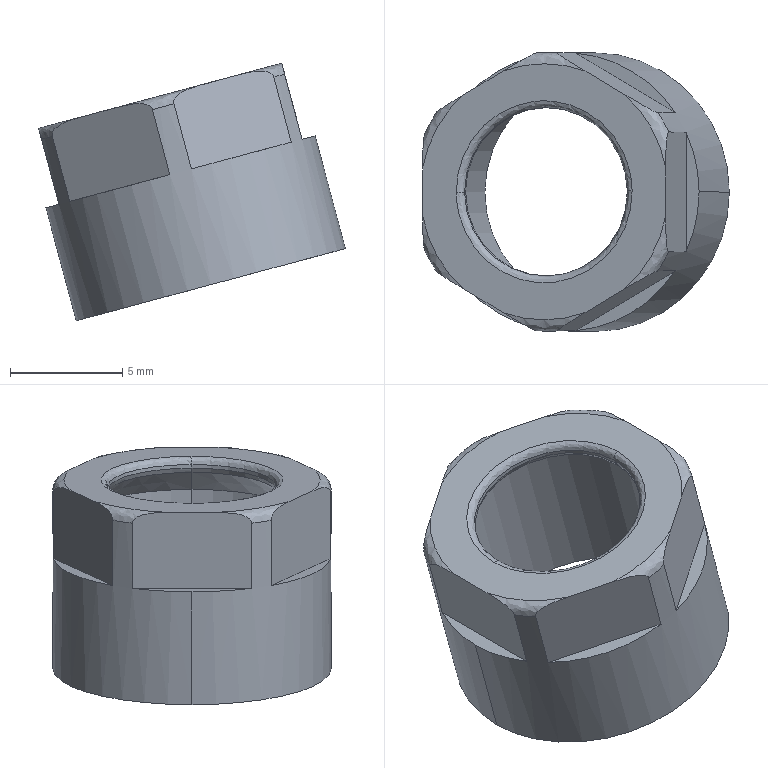Part | STEP file | _1-SO-96830001_1_1_1 | 1 solid | 32 faces | box 13.65 x 12.4 x 11.458 mm | volume 348.087 mm3 | plane 14 | spline 10 | cylinder 6 | cone 2 | commonest cylinder face diameters 7.5 x2 10.13 x2 12.4 x2